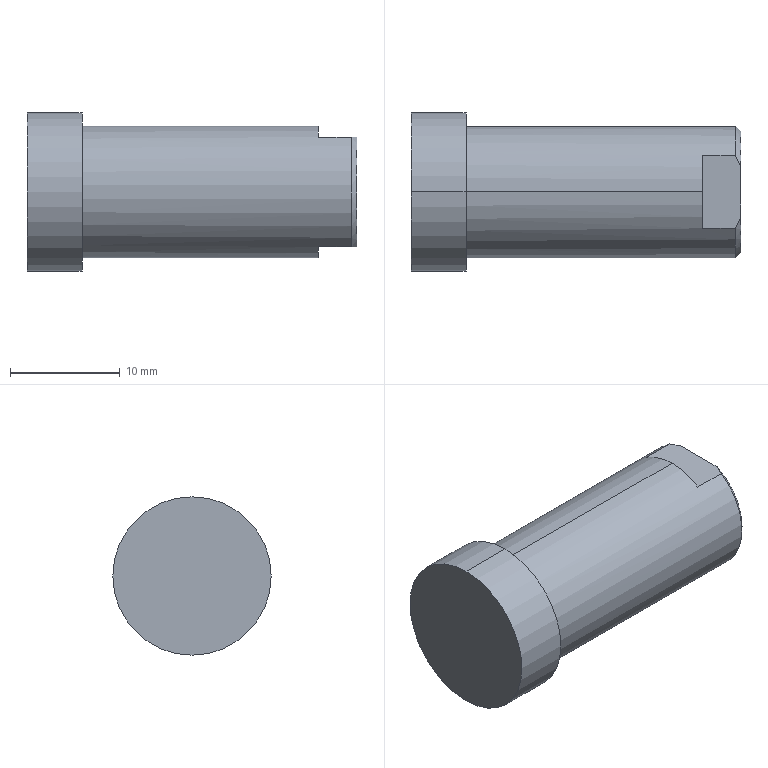Part | STEP file | _MSCCN25-15_rod_1 | 1 solid | 18 faces | box 30 x 14.4 x 14.4 mm | volume 3377 mm3 | plane 8 | cylinder 6 | cone 4 | commonest cylinder face diameters 4.917 x2 12 x2 14.4 x2
STEP:
#1=CARTESIAN_POINT('',(0.,0.,0.));
#2=DIRECTION('',(0.,0.,1.));
#3=DIRECTION('',(1.,0.,0.));
#4=AXIS2_PLACEMENT_3D('',#1,#2,#3);
#5=CARTESIAN_POINT('',(5.,0.,-6.));
#6=VERTEX_POINT('',#5);
#7=CARTESIAN_POINT('',(5.,0.,6.));
#8=VERTEX_POINT('',#7);
#9=CARTESIAN_POINT('',(5.,0.,0.));
#10=DIRECTION('',(1.,0.,0.));
#11=DIRECTION('',(0.,0.,-1.));
#12=AXIS2_PLACEMENT_3D('',#9,#10,#11);
#13=CIRCLE('',#12,6.);
#14=CARTESIAN_POINT('',(30.,0.,0.));
#15=DIRECTION('',(1.,0.,0.));
#16=DIRECTION('',(0.,0.,-1.));
#17=AXIS2_PLACEMENT_3D('',#14,#15,#16);
#18=CYLINDRICAL_SURFACE('',#17,6.);
#19=CARTESIAN_POINT('',(0.,-25.));
#20=DIRECTION('',(1.,0.));
#21=VECTOR('',#20,1.);
#22=LINE('',#19,#21);
#23=(GEOMETRIC_REPRESENTATION_CONTEXT(2)PARAMETRIC_REPRESENTATION_CONTEXT()REPRESENTATION_CONTEXT('',''));
#24=DEFINITIONAL_REPRESENTATION('',(#22),#23);
#25=PCURVE('',#18,#24);
#26=CARTESIAN_POINT('',(5.,7.2,0.));
#27=DIRECTION('',(-1.,0.,0.));
#28=DIRECTION('',(0.,0.,1.));
#29=AXIS2_PLACEMENT_3D('',#26,#27,#28);
#30=PLANE('',#29);
#31=CARTESIAN_POINT('',(-6.,-7.2));
#32=CARTESIAN_POINT('',(-6.,3.192));
#33=CARTESIAN_POINT('',(3.,-2.004));
#34=CARTESIAN_POINT('',(12.,-7.2));
#35=CARTESIAN_POINT('',(3.,-12.396));
#36=CARTESIAN_POINT('',(-6.,-17.592));
#37=CARTESIAN_POINT('',(-6.,-7.2));
#38=(BOUNDED_CURVE()B_SPLINE_CURVE(2,(#31,#32,#33,#34,#35,#36,#37),.UNSPECIFIED.,.T.,.F.)B_SPLINE_CURVE_WITH_KNOTS((1,2,2,2,2,1),(-2.094,0.,2.094,4.189,6.283,8.378),.UNSPECIFIED.)CURVE()GEOMETRIC_REPRESENTATION_ITEM()RATIONAL_B_SPLINE_CURVE((1.,0.5,1.,0.5,1.,0.5,1.))REPRESENTATION_ITEM(''));
#39=(GEOMETRIC_REPRESENTATION_CONTEXT(2)PARAMETRIC_REPRESENTATION_CONTEXT()REPRESENTATION_CONTEXT('',''));
#40=DEFINITIONAL_REPRESENTATION('',(#38),#39);
#41=PCURVE('',#30,#40);
#42=SURFACE_CURVE('',#13,(#25,#41),.PCURVE_S1.);
#43=EDGE_CURVE('',#6,#8,#42,.T.);
#44=ORIENTED_EDGE('',*,*,#43,.T.);
#45=CARTESIAN_POINT('',(26.5,0.,6.));
#46=VERTEX_POINT('',#45);
#47=CARTESIAN_POINT('',(30.,0.,6.));
#48=DIRECTION('',(1.,0.,0.));
#49=VECTOR('',#48,1.);
#50=LINE('',#47,#49);
#51=CARTESIAN_POINT('',(3.142,0.));
#52=DIRECTION('',(0.,1.));
#53=VECTOR('',#52,1.);
#54=LINE('',#51,#53);
#55=(GEOMETRIC_REPRESENTATION_CONTEXT(2)PARAMETRIC_REPRESENTATION_CONTEXT()REPRESENTATION_CONTEXT('',''));
#56=DEFINITIONAL_REPRESENTATION('',(#54),#55);
#57=PCURVE('',#18,#56);
#58=CARTESIAN_POINT('',(30.,0.,0.));
#59=DIRECTION('',(1.,0.,0.));
#60=DIRECTION('',(0.,0.,-1.));
#61=AXIS2_PLACEMENT_3D('',#58,#59,#60);
#62=CYLINDRICAL_SURFACE('',#61,6.);
#63=CARTESIAN_POINT('',(3.142,0.));
#64=DIRECTION('',(0.,1.));
#65=VECTOR('',#64,1.);
#66=LINE('',#63,#65);
#67=(GEOMETRIC_REPRESENTATION_CONTEXT(2)PARAMETRIC_REPRESENTATION_CONTEXT()REPRESENTATION_CONTEXT('',''));
#68=DEFINITIONAL_REPRESENTATION('',(#66),#67);
#69=PCURVE('',#62,#68);
#70=SURFACE_CURVE('',#50,(#57,#69),.PCURVE_S1.);
#71=EDGE_CURVE('',#8,#46,#70,.T.);
#72=ORIENTED_EDGE('',*,*,#71,.T.);
#73=CARTESIAN_POINT('',(26.5,3.317,5.));
#74=VERTEX_POINT('',#73);
#75=CARTESIAN_POINT('',(26.5,0.,0.));
#76=DIRECTION('',(-1.,0.,0.));
#77=DIRECTION('',(0.,0.,-1.));
#78=AXIS2_PLACEMENT_3D('',#75,#76,#77);
#79=CIRCLE('',#78,6.);
#80=CARTESIAN_POINT('',(6.283,-3.5));
#81=DIRECTION('',(-1.,0.));
#82=VECTOR('',#81,1.);
#83=LINE('',#80,#82);
#84=(GEOMETRIC_REPRESENTATION_CONTEXT(2)PARAMETRIC_REPRESENTATION_CONTEXT()REPRESENTATION_CONTEXT('',''));
#85=DEFINITIONAL_REPRESENTATION('',(#83),#84);
#86=PCURVE('',#18,#85);
#87=CARTESIAN_POINT('',(26.5,0.,0.));
#88=DIRECTION('',(1.,0.,0.));
#89=DIRECTION('',(0.,0.,-1.));
#90=AXIS2_PLACEMENT_3D('',#87,#88,#89);
#91=PLANE('',#90);
#92=CARTESIAN_POINT('',(6.,0.));
#93=CARTESIAN_POINT('',(6.,-10.392));
#94=CARTESIAN_POINT('',(-3.,-5.196));
#95=CARTESIAN_POINT('',(-12.,0.));
#96=CARTESIAN_POINT('',(-3.,5.196));
#97=CARTESIAN_POINT('',(6.,10.392));
#98=CARTESIAN_POINT('',(6.,0.));
#99=(BOUNDED_CURVE()B_SPLINE_CURVE(2,(#92,#93,#94,#95,#96,#97,#98),.UNSPECIFIED.,.T.,.F.)B_SPLINE_CURVE_WITH_KNOTS((1,2,2,2,2,1),(-2.094,0.,2.094,4.189,6.283,8.378),.UNSPECIFIED.)CURVE()GEOMETRIC_REPRESENTATION_ITEM()RATIONAL_B_SPLINE_CURVE((1.,0.5,1.,0.5,1.,0.5,1.))REPRESENTATION_ITEM(''));
#100=(GEOMETRIC_REPRESENTATION_CONTEXT(2)PARAMETRIC_REPRESENTATION_CONTEXT()REPRESENTATION_CONTEXT('',''));
#101=DEFINITIONAL_REPRESENTATION('',(#99),#100);
#102=PCURVE('',#91,#101);
#103=SURFACE_CURVE('',#79,(#86,#102),.PCURVE_S1.);
#104=EDGE_CURVE('',#46,#74,#103,.T.);
#105=ORIENTED_EDGE('',*,*,#104,.T.);
#106=CARTESIAN_POINT('',(29.5,3.317,5.));
#107=VERTEX_POINT('',#106);
#108=CARTESIAN_POINT('',(30.,3.317,5.));
#109=DIRECTION('',(1.,0.,0.));
#110=VECTOR('',#109,1.);
#111=LINE('',#108,#110);
#112=CARTESIAN_POINT('',(2.556,0.));
#113=DIRECTION('',(0.,1.));
#114=VECTOR('',#113,1.);
#115=LINE('',#112,#114);
#116=(GEOMETRIC_REPRESENTATION_CONTEXT(2)PARAMETRIC_REPRESENTATION_CONTEXT()REPRESENTATION_CONTEXT('',''));
#117=DEFINITIONAL_REPRESENTATION('',(#115),#116);
#118=PCURVE('',#18,#117);
#119=CARTESIAN_POINT('',(26.5,3.317,5.));
#120=DIRECTION('',(0.,0.,1.));
#121=DIRECTION('',(1.,0.,0.));
#122=AXIS2_PLACEMENT_3D('',#119,#120,#121);
#123=PLANE('',#122);
#124=CARTESIAN_POINT('',(3.5,0.));
#125=DIRECTION('',(1.,0.));
#126=VECTOR('',#125,1.);
#127=LINE('',#124,#126);
#128=(GEOMETRIC_REPRESENTATION_CONTEXT(2)PARAMETRIC_REPRESENTATION_CONTEXT()REPRESENTATION_CONTEXT('',''));
#129=DEFINITIONAL_REPRESENTATION('',(#127),#128);
#130=PCURVE('',#123,#129);
#131=SURFACE_CURVE('',#111,(#118,#130),.PCURVE_S1.);
#132=EDGE_CURVE('',#74,#107,#131,.T.);
#133=ORIENTED_EDGE('',*,*,#132,.T.);
#134=CARTESIAN_POINT('',(29.5,3.317,-5.));
#135=VERTEX_POINT('',#134);
#136=CARTESIAN_POINT('',(29.5,0.,0.));
#137=DIRECTION('',(-1.,0.,0.));
#138=DIRECTION('',(0.,0.,-1.));
#139=AXIS2_PLACEMENT_3D('',#136,#137,#138);
#140=CIRCLE('',#139,6.);
#141=CARTESIAN_POINT('',(6.283,-0.5));
#142=DIRECTION('',(-1.,0.));
#143=VECTOR('',#142,1.);
#144=LINE('',#141,#143);
#145=(GEOMETRIC_REPRESENTATION_CONTEXT(2)PARAMETRIC_REPRESENTATION_CONTEXT()REPRESENTATION_CONTEXT('',''));
#146=DEFINITIONAL_REPRESENTATION('',(#144),#145);
#147=PCURVE('',#18,#146);
#148=CARTESIAN_POINT('',(29.5,0.,0.));
#149=DIRECTION('',(-1.,0.,0.));
#150=DIRECTION('',(0.,0.,1.));
#151=AXIS2_PLACEMENT_3D('',#148,#149,#150);
#152=CONICAL_SURFACE('',#151,6.,0.7854);
#153=CARTESIAN_POINT('',(-3.142,0.));
#154=DIRECTION('',(1.,0.));
#155=VECTOR('',#154,1.);
#156=LINE('',#153,#155);
#157=(GEOMETRIC_REPRESENTATION_CONTEXT(2)PARAMETRIC_REPRESENTATION_CONTEXT()REPRESENTATION_CONTEXT('',''));
#158=DEFINITIONAL_REPRESENTATION('',(#156),#157);
#159=PCURVE('',#152,#158);
#160=SURFACE_CURVE('',#140,(#147,#159),.PCURVE_S1.);
#161=EDGE_CURVE('',#107,#135,#160,.T.);
#162=ORIENTED_EDGE('',*,*,#161,.T.);
#163=CARTESIAN_POINT('',(26.5,3.317,-5.));
#164=VERTEX_POINT('',#163);
#165=CARTESIAN_POINT('',(30.,3.317,-5.));
#166=DIRECTION('',(-1.,0.,0.));
#167=VECTOR('',#166,1.);
#168=LINE('',#165,#167);
#169=CARTESIAN_POINT('',(0.5857,0.));
#170=DIRECTION('',(0.,-1.));
#171=VECTOR('',#170,1.);
#172=LINE('',#169,#171);
#173=(GEOMETRIC_REPRESENTATION_CONTEXT(2)PARAMETRIC_REPRESENTATION_CONTEXT()REPRESENTATION_CONTEXT('',''));
#174=DEFINITIONAL_REPRESENTATION('',(#172),#173);
#175=PCURVE('',#18,#174);
#176=CARTESIAN_POINT('',(26.5,-3.317,-5.));
#177=DIRECTION('',(0.,0.,-1.));
#178=DIRECTION('',(-1.,0.,0.));
#179=AXIS2_PLACEMENT_3D('',#176,#177,#178);
#180=PLANE('',#179);
#181=CARTESIAN_POINT('',(-3.5,6.633));
#182=DIRECTION('',(1.,0.));
#183=VECTOR('',#182,1.);
#184=LINE('',#181,#183);
#185=(GEOMETRIC_REPRESENTATION_CONTEXT(2)PARAMETRIC_REPRESENTATION_CONTEXT()REPRESENTATION_CONTEXT('',''));
#186=DEFINITIONAL_REPRESENTATION('',(#184),#185);
#187=PCURVE('',#180,#186);
#188=SURFACE_CURVE('',#168,(#175,#187),.PCURVE_S1.);
#189=EDGE_CURVE('',#135,#164,#188,.T.);
#190=ORIENTED_EDGE('',*,*,#189,.T.);
#191=CARTESIAN_POINT('',(26.5,0.,-6.));
#192=VERTEX_POINT('',#191);
#193=CARTESIAN_POINT('',(26.5,0.,0.));
#194=DIRECTION('',(-1.,0.,0.));
#195=DIRECTION('',(0.,0.,-1.));
#196=AXIS2_PLACEMENT_3D('',#193,#194,#195);
#197=CIRCLE('',#196,6.);
#198=CARTESIAN_POINT('',(6.283,-3.5));
#199=DIRECTION('',(-1.,0.));
#200=VECTOR('',#199,1.);
#201=LINE('',#198,#200);
#202=(GEOMETRIC_REPRESENTATION_CONTEXT(2)PARAMETRIC_REPRESENTATION_CONTEXT()REPRESENTATION_CONTEXT('',''));
#203=DEFINITIONAL_REPRESENTATION('',(#201),#202);
#204=PCURVE('',#18,#203);
#205=CARTESIAN_POINT('',(26.5,0.,0.));
#206=DIRECTION('',(1.,0.,0.));
#207=DIRECTION('',(0.,0.,-1.));
#208=AXIS2_PLACEMENT_3D('',#205,#206,#207);
#209=PLANE('',#208);
#210=CARTESIAN_POINT('',(6.,0.));
#211=CARTESIAN_POINT('',(6.,-10.392));
#212=CARTESIAN_POINT('',(-3.,-5.196));
#213=CARTESIAN_POINT('',(-12.,0.));
#214=CARTESIAN_POINT('',(-3.,5.196));
#215=CARTESIAN_POINT('',(6.,10.392));
#216=CARTESIAN_POINT('',(6.,0.));
#217=(BOUNDED_CURVE()B_SPLINE_CURVE(2,(#210,#211,#212,#213,#214,#215,#216),.UNSPECIFIED.,.T.,.F.)B_SPLINE_CURVE_WITH_KNOTS((1,2,2,2,2,1),(-2.094,0.,2.094,4.189,6.283,8.378),.UNSPECIFIED.)CURVE()GEOMETRIC_REPRESENTATION_ITEM()RATIONAL_B_SPLINE_CURVE((1.,0.5,1.,0.5,1.,0.5,1.))REPRESENTATION_ITEM(''));
#218=(GEOMETRIC_REPRESENTATION_CONTEXT(2)PARAMETRIC_REPRESENTATION_CONTEXT()REPRESENTATION_CONTEXT('',''));
#219=DEFINITIONAL_REPRESENTATION('',(#217),#218);
#220=PCURVE('',#209,#219);
#221=SURFACE_CURVE('',#197,(#204,#220),.PCURVE_S1.);
#222=EDGE_CURVE('',#164,#192,#221,.T.);
#223=ORIENTED_EDGE('',*,*,#222,.T.);
#224=CARTESIAN_POINT('',(30.,0.,-6.));
#225=DIRECTION('',(1.,0.,0.));
#226=VECTOR('',#225,1.);
#227=LINE('',#224,#226);
#228=CARTESIAN_POINT('',(0.,0.));
#229=DIRECTION('',(0.,1.));
#230=VECTOR('',#229,1.);
#231=LINE('',#228,#230);
#232=(GEOMETRIC_REPRESENTATION_CONTEXT(2)PARAMETRIC_REPRESENTATION_CONTEXT()REPRESENTATION_CONTEXT('',''));
#233=DEFINITIONAL_REPRESENTATION('',(#231),#232);
#234=PCURVE('',#18,#233);
#235=CARTESIAN_POINT('',(6.283,0.));
#236=DIRECTION('',(0.,1.));
#237=VECTOR('',#236,1.);
#238=LINE('',#235,#237);
#239=(GEOMETRIC_REPRESENTATION_CONTEXT(2)PARAMETRIC_REPRESENTATION_CONTEXT()REPRESENTATION_CONTEXT('',''));
#240=DEFINITIONAL_REPRESENTATION('',(#238),#239);
#241=PCURVE('',#62,#240);
#242=SURFACE_CURVE('',#227,(#234,#241),.PCURVE_S1.);
#243=EDGE_CURVE('',#6,#192,#242,.T.);
#244=ORIENTED_EDGE('',*,*,#243,.F.);
#245=EDGE_LOOP('',(#44,#72,#105,#133,#162,#190,#223,#244));
#246=FACE_BOUND('',#245,.T.);
#247=ADVANCED_FACE('',(#246),#18,.T.);
#248=CARTESIAN_POINT('',(0.,0.,-7.2));
#249=VERTEX_POINT('',#248);
#250=CARTESIAN_POINT('',(0.,0.,7.2));
#251=VERTEX_POINT('',#250);
#252=CARTESIAN_POINT('',(0.,0.,0.));
#253=DIRECTION('',(1.,0.,0.));
#254=DIRECTION('',(0.,0.,-1.));
#255=AXIS2_PLACEMENT_3D('',#252,#253,#254);
#256=CIRCLE('',#255,7.2);
#257=CARTESIAN_POINT('',(30.,0.,0.));
#258=DIRECTION('',(1.,0.,0.));
#259=DIRECTION('',(0.,0.,-1.));
#260=AXIS2_PLACEMENT_3D('',#257,#258,#259);
#261=CYLINDRICAL_SURFACE('',#260,7.2);
#262=CARTESIAN_POINT('',(0.,-30.));
#263=DIRECTION('',(1.,0.));
#264=VECTOR('',#263,1.);
#265=LINE('',#262,#264);
#266=(GEOMETRIC_REPRESENTATION_CONTEXT(2)PARAMETRIC_REPRESENTATION_CONTEXT()REPRESENTATION_CONTEXT('',''));
#267=DEFINITIONAL_REPRESENTATION('',(#265),#266);
#268=PCURVE('',#261,#267);
#269=CARTESIAN_POINT('',(0.,0.,0.));
#270=DIRECTION('',(1.,0.,0.));
#271=DIRECTION('',(0.,0.,-1.));
#272=AXIS2_PLACEMENT_3D('',#269,#270,#271);
#273=PLANE('',#272);
#274=CARTESIAN_POINT('',(0.,0.));
#275=DIRECTION('',(1.,0.));
#276=AXIS2_PLACEMENT_2D('',#274,#275);
#277=CIRCLE('',#276,7.2);
#278=(GEOMETRIC_REPRESENTATION_CONTEXT(2)PARAMETRIC_REPRESENTATION_CONTEXT()REPRESENTATION_CONTEXT('',''));
#279=DEFINITIONAL_REPRESENTATION('',(#277),#278);
#280=PCURVE('',#273,#279);
#281=SURFACE_CURVE('',#256,(#268,#280),.PCURVE_S1.);
#282=EDGE_CURVE('',#249,#251,#281,.T.);
#283=ORIENTED_EDGE('',*,*,#282,.T.);
#284=CARTESIAN_POINT('',(5.,0.,7.2));
#285=VERTEX_POINT('',#284);
#286=CARTESIAN_POINT('',(30.,0.,7.2));
#287=DIRECTION('',(1.,0.,0.));
#288=VECTOR('',#287,1.);
#289=LINE('',#286,#288);
#290=CARTESIAN_POINT('',(3.142,0.));
#291=DIRECTION('',(0.,1.));
#292=VECTOR('',#291,1.);
#293=LINE('',#290,#292);
#294=(GEOMETRIC_REPRESENTATION_CONTEXT(2)PARAMETRIC_REPRESENTATION_CONTEXT()REPRESENTATION_CONTEXT('',''));
#295=DEFINITIONAL_REPRESENTATION('',(#293),#294);
#296=PCURVE('',#261,#295);
#297=CARTESIAN_POINT('',(30.,0.,0.));
#298=DIRECTION('',(1.,0.,0.));
#299=DIRECTION('',(0.,0.,-1.));
#300=AXIS2_PLACEMENT_3D('',#297,#298,#299);
#301=CYLINDRICAL_SURFACE('',#300,7.2);
#302=CARTESIAN_POINT('',(3.142,0.));
#303=DIRECTION('',(0.,1.));
#304=VECTOR('',#303,1.);
#305=LINE('',#302,#304);
#306=(GEOMETRIC_REPRESENTATION_CONTEXT(2)PARAMETRIC_REPRESENTATION_CONTEXT()REPRESENTATION_CONTEXT('',''));
#307=DEFINITIONAL_REPRESENTATION('',(#305),#306);
#308=PCURVE('',#301,#307);
#309=SURFACE_CURVE('',#289,(#296,#308),.PCURVE_S1.);
#310=EDGE_CURVE('',#251,#285,#309,.T.);
#311=ORIENTED_EDGE('',*,*,#310,.T.);
#312=CARTESIAN_POINT('',(5.,0.,-7.2));
#313=VERTEX_POINT('',#312);
#314=CARTESIAN_POINT('',(5.,0.,0.));
#315=DIRECTION('',(-1.,0.,0.));
#316=DIRECTION('',(0.,0.,-1.));
#317=AXIS2_PLACEMENT_3D('',#314,#315,#316);
#318=CIRCLE('',#317,7.2);
#319=CARTESIAN_POINT('',(6.283,-25.));
#320=DIRECTION('',(-1.,0.));
#321=VECTOR('',#320,1.);
#322=LINE('',#319,#321);
#323=(GEOMETRIC_REPRESENTATION_CONTEXT(2)PARAMETRIC_REPRESENTATION_CONTEXT()REPRESENTATION_CONTEXT('',''));
#324=DEFINITIONAL_REPRESENTATION('',(#322),#323);
#325=PCURVE('',#261,#324);
#326=CARTESIAN_POINT('',(0.,-7.2));
#327=DIRECTION('',(-1.,0.));
#328=AXIS2_PLACEMENT_2D('',#326,#327);
#329=CIRCLE('',#328,7.2);
#330=(GEOMETRIC_REPRESENTATION_CONTEXT(2)PARAMETRIC_REPRESENTATION_CONTEXT()REPRESENTATION_CONTEXT('',''));
#331=DEFINITIONAL_REPRESENTATION('',(#329),#330);
#332=PCURVE('',#30,#331);
#333=SURFACE_CURVE('',#318,(#325,#332),.PCURVE_S1.);
#334=EDGE_CURVE('',#285,#313,#333,.T.);
#335=ORIENTED_EDGE('',*,*,#334,.T.);
#336=CARTESIAN_POINT('',(30.,0.,-7.2));
#337=DIRECTION('',(1.,0.,0.));
#338=VECTOR('',#337,1.);
#339=LINE('',#336,#338);
#340=CARTESIAN_POINT('',(0.,0.));
#341=DIRECTION('',(0.,1.));
#342=VECTOR('',#341,1.);
#343=LINE('',#340,#342);
#344=(GEOMETRIC_REPRESENTATION_CONTEXT(2)PARAMETRIC_REPRESENTATION_CONTEXT()REPRESENTATION_CONTEXT('',''));
#345=DEFINITIONAL_REPRESENTATION('',(#343),#344);
#346=PCURVE('',#261,#345);
#347=CARTESIAN_POINT('',(6.283,0.));
#348=DIRECTION('',(0.,1.));
#349=VECTOR('',#348,1.);
#350=LINE('',#347,#349);
#351=(GEOMETRIC_REPRESENTATION_CONTEXT(2)PARAMETRIC_REPRESENTATION_CONTEXT()REPRESENTATION_CONTEXT('',''));
#352=DEFINITIONAL_REPRESENTATION('',(#350),#351);
#353=PCURVE('',#301,#352);
#354=SURFACE_CURVE('',#339,(#346,#353),.PCURVE_S1.);
#355=EDGE_CURVE('',#249,#313,#354,.T.);
#356=ORIENTED_EDGE('',*,*,#355,.F.);
#357=EDGE_LOOP('',(#283,#311,#335,#356));
#358=FACE_BOUND('',#357,.T.);
#359=ADVANCED_FACE('',(#358),#261,.T.);
#360=CARTESIAN_POINT('',(29.459,0.,-2.458));
#361=VERTEX_POINT('',#360);
#362=CARTESIAN_POINT('',(29.459,2.458,0.));
#363=VERTEX_POINT('',#362);
#364=CARTESIAN_POINT('',(29.459,0.,0.));
#365=DIRECTION('',(1.,0.,0.));
#366=DIRECTION('',(0.,0.,-1.));
#367=AXIS2_PLACEMENT_3D('',#364,#365,#366);
#368=CIRCLE('',#367,2.458);
#369=CARTESIAN_POINT('',(30.,0.,0.));
#370=DIRECTION('',(1.,0.,0.));
#371=DIRECTION('',(0.,1.,0.));
#372=AXIS2_PLACEMENT_3D('',#369,#370,#371);
#373=CONICAL_SURFACE('',#372,3.,0.7854);
#374=CARTESIAN_POINT('',(4.712,-0.5415));
#375=DIRECTION('',(1.,0.));
#376=VECTOR('',#375,1.);
#377=LINE('',#374,#376);
#378=(GEOMETRIC_REPRESENTATION_CONTEXT(2)PARAMETRIC_REPRESENTATION_CONTEXT()REPRESENTATION_CONTEXT('',''));
#379=DEFINITIONAL_REPRESENTATION('',(#377),#378);
#380=PCURVE('',#373,#379);
#381=CARTESIAN_POINT('',(30.,0.,0.));
#382=DIRECTION('',(1.,0.,0.));
#383=DIRECTION('',(0.,0.,-1.));
#384=AXIS2_PLACEMENT_3D('',#381,#382,#383);
#385=CYLINDRICAL_SURFACE('',#384,2.458);
#386=CARTESIAN_POINT('',(0.,-0.5415));
#387=DIRECTION('',(1.,0.));
#388=VECTOR('',#387,1.);
#389=LINE('',#386,#388);
#390=(GEOMETRIC_REPRESENTATION_CONTEXT(2)PARAMETRIC_REPRESENTATION_CONTEXT()REPRESENTATION_CONTEXT('',''));
#391=DEFINITIONAL_REPRESENTATION('',(#389),#390);
#392=PCURVE('',#385,#391);
#393=SURFACE_CURVE('',#368,(#380,#392),.PCURVE_S1.);
#394=EDGE_CURVE('',#361,#363,#393,.T.);
#395=ORIENTED_EDGE('',*,*,#394,.T.);
#396=CARTESIAN_POINT('',(30.,3.,0.));
#397=VERTEX_POINT('',#396);
#398=CARTESIAN_POINT('',(30.,3.,0.));
#399=DIRECTION('',(0.7071,0.7071,0.));
#400=VECTOR('',#399,1.);
#401=LINE('',#398,#400);
#402=CARTESIAN_POINT('',(6.283,0.));
#403=DIRECTION('',(0.,1.));
#404=VECTOR('',#403,1.);
#405=LINE('',#402,#404);
#406=(GEOMETRIC_REPRESENTATION_CONTEXT(2)PARAMETRIC_REPRESENTATION_CONTEXT()REPRESENTATION_CONTEXT('',''));
#407=DEFINITIONAL_REPRESENTATION('',(#405),#406);
#408=PCURVE('',#373,#407);
#409=CARTESIAN_POINT('',(30.,0.,0.));
#410=DIRECTION('',(1.,0.,0.));
#411=DIRECTION('',(0.,1.,0.));
#412=AXIS2_PLACEMENT_3D('',#409,#410,#411);
#413=CONICAL_SURFACE('',#412,3.,0.7854);
#414=CARTESIAN_POINT('',(0.,0.));
#415=DIRECTION('',(0.,1.));
#416=VECTOR('',#415,1.);
#417=LINE('',#414,#416);
#418=(GEOMETRIC_REPRESENTATION_CONTEXT(2)PARAMETRIC_REPRESENTATION_CONTEXT()REPRESENTATION_CONTEXT('',''));
#419=DEFINITIONAL_REPRESENTATION('',(#417),#418);
#420=PCURVE('',#413,#419);
#421=SURFACE_CURVE('',#401,(#408,#420),.PCURVE_S1.);
#422=EDGE_CURVE('',#363,#397,#421,.T.);
#423=ORIENTED_EDGE('',*,*,#422,.T.);
#424=CARTESIAN_POINT('',(30.,-3.,0.));
#425=VERTEX_POINT('',#424);
#426=CARTESIAN_POINT('',(30.,0.,0.));
#427=DIRECTION('',(1.,0.,0.));
#428=DIRECTION('',(0.,1.,0.));
#429=AXIS2_PLACEMENT_3D('',#426,#427,#428);
#430=CIRCLE('',#429,3.);
#431=CARTESIAN_POINT('',(0.,0.));
#432=DIRECTION('',(1.,0.));
#433=VECTOR('',#432,1.);
#434=LINE('',#431,#433);
#435=(GEOMETRIC_REPRESENTATION_CONTEXT(2)PARAMETRIC_REPRESENTATION_CONTEXT()REPRESENTATION_CONTEXT('',''));
#436=DEFINITIONAL_REPRESENTATION('',(#434),#435);
#437=PCURVE('',#373,#436);
#438=CARTESIAN_POINT('',(30.,5.5,0.));
#439=DIRECTION('',(-1.,0.,0.));
#440=DIRECTION('',(0.,0.,1.));
#441=AXIS2_PLACEMENT_3D('',#438,#439,#440);
#442=PLANE('',#441);
#443=CARTESIAN_POINT('',(0.,-2.5));
#444=CARTESIAN_POINT('',(5.196,-2.5));
#445=CARTESIAN_POINT('',(2.598,-7.));
#446=CARTESIAN_POINT('',(0.,-11.5));
#447=CARTESIAN_POINT('',(-2.598,-7.));
#448=CARTESIAN_POINT('',(-5.196,-2.5));
#449=CARTESIAN_POINT('',(0.,-2.5));
#450=(BOUNDED_CURVE()B_SPLINE_CURVE(2,(#443,#444,#445,#446,#447,#448,#449),.UNSPECIFIED.,.T.,.F.)B_SPLINE_CURVE_WITH_KNOTS((1,2,2,2,2,1),(-2.094,0.,2.094,4.189,6.283,8.378),.UNSPECIFIED.)CURVE()GEOMETRIC_REPRESENTATION_ITEM()RATIONAL_B_SPLINE_CURVE((1.,0.5,1.,0.5,1.,0.5,1.))REPRESENTATION_ITEM(''));
#451=(GEOMETRIC_REPRESENTATION_CONTEXT(2)PARAMETRIC_REPRESENTATION_CONTEXT()REPRESENTATION_CONTEXT('',''));
#452=DEFINITIONAL_REPRESENTATION('',(#450),#451);
#453=PCURVE('',#442,#452);
#454=SURFACE_CURVE('',#430,(#437,#453),.PCURVE_S1.);
#455=EDGE_CURVE('',#425,#397,#454,.T.);
#456=ORIENTED_EDGE('',*,*,#455,.F.);
#457=CARTESIAN_POINT('',(29.459,-2.458,0.));
#458=VERTEX_POINT('',#457);
#459=CARTESIAN_POINT('',(30.,-3.,0.));
#460=DIRECTION('',(0.7071,-0.7071,0.));
#461=VECTOR('',#460,1.);
#462=LINE('',#459,#461);
#463=CARTESIAN_POINT('',(3.142,0.));
#464=DIRECTION('',(0.,1.));
#465=VECTOR('',#464,1.);
#466=LINE('',#463,#465);
#467=(GEOMETRIC_REPRESENTATION_CONTEXT(2)PARAMETRIC_REPRESENTATION_CONTEXT()REPRESENTATION_CONTEXT('',''));
#468=DEFINITIONAL_REPRESENTATION('',(#466),#467);
#469=PCURVE('',#373,#468);
#470=CARTESIAN_POINT('',(3.142,0.));
#471=DIRECTION('',(0.,1.));
#472=VECTOR('',#471,1.);
#473=LINE('',#470,#472);
#474=(GEOMETRIC_REPRESENTATION_CONTEXT(2)PARAMETRIC_REPRESENTATION_CONTEXT()REPRESENTATION_CONTEXT('',''));
#475=DEFINITIONAL_REPRESENTATION('',(#473),#474);
#476=PCURVE('',#413,#475);
#477=SURFACE_CURVE('',#462,(#469,#476),.PCURVE_S1.);
#478=EDGE_CURVE('',#458,#425,#477,.T.);
#479=ORIENTED_EDGE('',*,*,#478,.F.);
#480=CARTESIAN_POINT('',(29.459,0.,0.));
#481=DIRECTION('',(1.,0.,0.));
#482=DIRECTION('',(0.,0.,-1.));
#483=AXIS2_PLACEMENT_3D('',#480,#481,#482);
#484=CIRCLE('',#483,2.458);
#485=CARTESIAN_POINT('',(-1.571,-0.5415));
#486=DIRECTION('',(1.,0.));
#487=VECTOR('',#486,1.);
#488=LINE('',#485,#487);
#489=(GEOMETRIC_REPRESENTATION_CONTEXT(2)PARAMETRIC_REPRESENTATION_CONTEXT()REPRESENTATION_CONTEXT('',''));
#490=DEFINITIONAL_REPRESENTATION('',(#488),#489);
#491=PCURVE('',#373,#490);
#492=CARTESIAN_POINT('',(30.,0.,0.));
#493=DIRECTION('',(1.,0.,0.));
#494=DIRECTION('',(0.,0.,-1.));
#495=AXIS2_PLACEMENT_3D('',#492,#493,#494);
#496=CYLINDRICAL_SURFACE('',#495,2.458);
#497=CARTESIAN_POINT('',(0.,-0.5415));
#498=DIRECTION('',(1.,0.));
#499=VECTOR('',#498,1.);
#500=LINE('',#497,#499);
#501=(GEOMETRIC_REPRESENTATION_CONTEXT(2)PARAMETRIC_REPRESENTATION_CONTEXT()REPRESENTATION_CONTEXT('',''));
#502=DEFINITIONAL_REPRESENTATION('',(#500),#501);
#503=PCURVE('',#496,#502);
#504=SURFACE_CURVE('',#484,(#491,#503),.PCURVE_S1.);
#505=EDGE_CURVE('',#458,#361,#504,.T.);
#506=ORIENTED_EDGE('',*,*,#505,.T.);
#507=EDGE_LOOP('',(#395,#423,#456,#479,#506));
#508=FACE_BOUND('',#507,.F.);
#509=ADVANCED_FACE('',(#508),#373,.F.);
#510=CARTESIAN_POINT('',(18.,0.,-2.458));
#511=VERTEX_POINT('',#510);
#512=CARTESIAN_POINT('',(30.,0.,-2.458));
#513=DIRECTION('',(1.,0.,0.));
#514=VECTOR('',#513,1.);
#515=LINE('',#512,#514);
#516=CARTESIAN_POINT('',(6.283,0.));
#517=DIRECTION('',(0.,1.));
#518=VECTOR('',#517,1.);
#519=LINE('',#516,#518);
#520=(GEOMETRIC_REPRESENTATION_CONTEXT(2)PARAMETRIC_REPRESENTATION_CONTEXT()REPRESENTATION_CONTEXT('',''));
#521=DEFINITIONAL_REPRESENTATION('',(#519),#520);
#522=PCURVE('',#496,#521);
#523=CARTESIAN_POINT('',(0.,0.));
#524=DIRECTION('',(0.,1.));
#525=VECTOR('',#524,1.);
#526=LINE('',#523,#525);
#527=(GEOMETRIC_REPRESENTATION_CONTEXT(2)PARAMETRIC_REPRESENTATION_CONTEXT()REPRESENTATION_CONTEXT('',''));
#528=DEFINITIONAL_REPRESENTATION('',(#526),#527);
#529=PCURVE('',#385,#528);
#530=SURFACE_CURVE('',#515,(#522,#529),.PCURVE_S1.);
#531=EDGE_CURVE('',#511,#361,#530,.T.);
#532=ORIENTED_EDGE('',*,*,#531,.T.);
#533=ORIENTED_EDGE('',*,*,#505,.F.);
#534=CARTESIAN_POINT('',(29.459,0.,2.458));
#535=VERTEX_POINT('',#534);
#536=CARTESIAN_POINT('',(29.459,0.,0.));
#537=DIRECTION('',(1.,0.,0.));
#538=DIRECTION('',(0.,0.,-1.));
#539=AXIS2_PLACEMENT_3D('',#536,#537,#538);
#540=CIRCLE('',#539,2.458);
#541=CARTESIAN_POINT('',(0.,-0.5415));
#542=DIRECTION('',(1.,0.));
#543=VECTOR('',#542,1.);
#544=LINE('',#541,#543);
#545=(GEOMETRIC_REPRESENTATION_CONTEXT(2)PARAMETRIC_REPRESENTATION_CONTEXT()REPRESENTATION_CONTEXT('',''));
#546=DEFINITIONAL_REPRESENTATION('',(#544),#545);
#547=PCURVE('',#496,#546);
#548=CARTESIAN_POINT('',(-1.571,-0.5415));
#549=DIRECTION('',(1.,0.));
#550=VECTOR('',#549,1.);
#551=LINE('',#548,#550);
#552=(GEOMETRIC_REPRESENTATION_CONTEXT(2)PARAMETRIC_REPRESENTATION_CONTEXT()REPRESENTATION_CONTEXT('',''));
#553=DEFINITIONAL_REPRESENTATION('',(#551),#552);
#554=PCURVE('',#413,#553);
#555=SURFACE_CURVE('',#540,(#547,#554),.PCURVE_S1.);
#556=EDGE_CURVE('',#535,#458,#555,.T.);
#557=ORIENTED_EDGE('',*,*,#556,.F.);
#558=CARTESIAN_POINT('',(18.,0.,2.458));
#559=VERTEX_POINT('',#558);
#560=CARTESIAN_POINT('',(30.,0.,2.458));
#561=DIRECTION('',(1.,0.,0.));
#562=VECTOR('',#561,1.);
#563=LINE('',#560,#562);
#564=CARTESIAN_POINT('',(3.142,0.));
#565=DIRECTION('',(0.,1.));
#566=VECTOR('',#565,1.);
#567=LINE('',#564,#566);
#568=(GEOMETRIC_REPRESENTATION_CONTEXT(2)PARAMETRIC_REPRESENTATION_CONTEXT()REPRESENTATION_CONTEXT('',''));
#569=DEFINITIONAL_REPRESENTATION('',(#567),#568);
#570=PCURVE('',#496,#569);
#571=CARTESIAN_POINT('',(3.142,0.));
#572=DIRECTION('',(0.,1.));
#573=VECTOR('',#572,1.);
#574=LINE('',#571,#573);
#575=(GEOMETRIC_REPRESENTATION_CONTEXT(2)PARAMETRIC_REPRESENTATION_CONTEXT()REPRESENTATION_CONTEXT('',''));
#576=DEFINITIONAL_REPRESENTATION('',(#574),#575);
#577=PCURVE('',#385,#576);
#578=SURFACE_CURVE('',#563,(#570,#577),.PCURVE_S1.);
#579=EDGE_CURVE('',#559,#535,#578,.T.);
#580=ORIENTED_EDGE('',*,*,#579,.F.);
#581=CARTESIAN_POINT('',(18.,0.,0.));
#582=DIRECTION('',(1.,0.,0.));
#583=DIRECTION('',(0.,0.,-1.));
#584=AXIS2_PLACEMENT_3D('',#581,#582,#583);
#585=CIRCLE('',#584,2.458);
#586=CARTESIAN_POINT('',(0.,-12.));
#587=DIRECTION('',(1.,0.));
#588=VECTOR('',#587,1.);
#589=LINE('',#586,#588);
#590=(GEOMETRIC_REPRESENTATION_CONTEXT(2)PARAMETRIC_REPRESENTATION_CONTEXT()REPRESENTATION_CONTEXT('',''));
#591=DEFINITIONAL_REPRESENTATION('',(#589),#590);
#592=PCURVE('',#496,#591);
#593=CARTESIAN_POINT('',(18.,0.,0.));
#594=DIRECTION('',(1.,0.,0.));
#595=DIRECTION('',(0.,0.,-1.));
#596=AXIS2_PLACEMENT_3D('',#593,#594,#595);
#597=PLANE('',#596);
#598=CARTESIAN_POINT('',(0.,0.));
#599=DIRECTION('',(1.,0.));
#600=AXIS2_PLACEMENT_2D('',#598,#599);
#601=CIRCLE('',#600,2.458);
#602=(GEOMETRIC_REPRESENTATION_CONTEXT(2)PARAMETRIC_REPRESENTATION_CONTEXT()REPRESENTATION_CONTEXT('',''));
#603=DEFINITIONAL_REPRESENTATION('',(#601),#602);
#604=PCURVE('',#597,#603);
#605=SURFACE_CURVE('',#585,(#592,#604),.PCURVE_S1.);
#606=EDGE_CURVE('',#559,#511,#605,.T.);
#607=ORIENTED_EDGE('',*,*,#606,.T.);
#608=EDGE_LOOP('',(#532,#533,#557,#580,#607));
#609=FACE_BOUND('',#608,.F.);
#610=ADVANCED_FACE('',(#609),#496,.F.);
#611=ORIENTED_EDGE('',*,*,#71,.F.);
#612=CARTESIAN_POINT('',(5.,0.,0.));
#613=DIRECTION('',(1.,0.,0.));
#614=DIRECTION('',(0.,0.,-1.));
#615=AXIS2_PLACEMENT_3D('',#612,#613,#614);
#616=CIRCLE('',#615,6.);
#617=CARTESIAN_POINT('',(0.,-25.));
#618=DIRECTION('',(1.,0.));
#619=VECTOR('',#618,1.);
#620=LINE('',#617,#619);
#621=(GEOMETRIC_REPRESENTATION_CONTEXT(2)PARAMETRIC_REPRESENTATION_CONTEXT()REPRESENTATION_CONTEXT('',''));
#622=DEFINITIONAL_REPRESENTATION('',(#620),#621);
#623=PCURVE('',#62,#622);
#624=CARTESIAN_POINT('',(-6.,-7.2));
#625=CARTESIAN_POINT('',(-6.,3.192));
#626=CARTESIAN_POINT('',(3.,-2.004));
#627=CARTESIAN_POINT('',(12.,-7.2));
#628=CARTESIAN_POINT('',(3.,-12.396));
#629=CARTESIAN_POINT('',(-6.,-17.592));
#630=CARTESIAN_POINT('',(-6.,-7.2));
#631=(BOUNDED_CURVE()B_SPLINE_CURVE(2,(#624,#625,#626,#627,#628,#629,#630),.UNSPECIFIED.,.T.,.F.)B_SPLINE_CURVE_WITH_KNOTS((1,2,2,2,2,1),(-2.094,0.,2.094,4.189,6.283,8.378),.UNSPECIFIED.)CURVE()GEOMETRIC_REPRESENTATION_ITEM()RATIONAL_B_SPLINE_CURVE((1.,0.5,1.,0.5,1.,0.5,1.))REPRESENTATION_ITEM(''));
#632=(GEOMETRIC_REPRESENTATION_CONTEXT(2)PARAMETRIC_REPRESENTATION_CONTEXT()REPRESENTATION_CONTEXT('',''));
#633=DEFINITIONAL_REPRESENTATION('',(#631),#632);
#634=PCURVE('',#30,#633);
#635=SURFACE_CURVE('',#616,(#623,#634),.PCURVE_S1.);
#636=EDGE_CURVE('',#8,#6,#635,.T.);
#637=ORIENTED_EDGE('',*,*,#636,.T.);
#638=ORIENTED_EDGE('',*,*,#243,.T.);
#639=CARTESIAN_POINT('',(26.5,-3.317,-5.));
#640=VERTEX_POINT('',#639);
#641=CARTESIAN_POINT('',(26.5,0.,0.));
#642=DIRECTION('',(-1.,0.,0.));
#643=DIRECTION('',(0.,0.,-1.));
#644=AXIS2_PLACEMENT_3D('',#641,#642,#643);
#645=CIRCLE('',#644,6.);
#646=CARTESIAN_POINT('',(6.283,-3.5));
#647=DIRECTION('',(-1.,0.));
#648=VECTOR('',#647,1.);
#649=LINE('',#646,#648);
#650=(GEOMETRIC_REPRESENTATION_CONTEXT(2)PARAMETRIC_REPRESENTATION_CONTEXT()REPRESENTATION_CONTEXT('',''));
#651=DEFINITIONAL_REPRESENTATION('',(#649),#650);
#652=PCURVE('',#62,#651);
#653=CARTESIAN_POINT('',(6.,0.));
#654=CARTESIAN_POINT('',(6.,-10.392));
#655=CARTESIAN_POINT('',(-3.,-5.196));
#656=CARTESIAN_POINT('',(-12.,0.));
#657=CARTESIAN_POINT('',(-3.,5.196));
#658=CARTESIAN_POINT('',(6.,10.392));
#659=CARTESIAN_POINT('',(6.,0.));
#660=(BOUNDED_CURVE()B_SPLINE_CURVE(2,(#653,#654,#655,#656,#657,#658,#659),.UNSPECIFIED.,.T.,.F.)B_SPLINE_CURVE_WITH_KNOTS((1,2,2,2,2,1),(-2.094,0.,2.094,4.189,6.283,8.378),.UNSPECIFIED.)CURVE()GEOMETRIC_REPRESENTATION_ITEM()RATIONAL_B_SPLINE_CURVE((1.,0.5,1.,0.5,1.,0.5,1.))REPRESENTATION_ITEM(''));
#661=(GEOMETRIC_REPRESENTATION_CONTEXT(2)PARAMETRIC_REPRESENTATION_CONTEXT()REPRESENTATION_CONTEXT('',''));
#662=DEFINITIONAL_REPRESENTATION('',(#660),#661);
#663=PCURVE('',#209,#662);
#664=SURFACE_CURVE('',#645,(#652,#663),.PCURVE_S1.);
#665=EDGE_CURVE('',#192,#640,#664,.T.);
#666=ORIENTED_EDGE('',*,*,#665,.T.);
#667=CARTESIAN_POINT('',(29.5,-3.317,-5.));
#668=VERTEX_POINT('',#667);
#669=CARTESIAN_POINT('',(30.,-3.317,-5.));
#670=DIRECTION('',(1.,0.,0.));
#671=VECTOR('',#670,1.);
#672=LINE('',#669,#671);
#673=CARTESIAN_POINT('',(5.697,0.));
#674=DIRECTION('',(0.,1.));
#675=VECTOR('',#674,1.);
#676=LINE('',#673,#675);
#677=(GEOMETRIC_REPRESENTATION_CONTEXT(2)PARAMETRIC_REPRESENTATION_CONTEXT()REPRESENTATION_CONTEXT('',''));
#678=DEFINITIONAL_REPRESENTATION('',(#676),#677);
#679=PCURVE('',#62,#678);
#680=CARTESIAN_POINT('',(-3.5,0.));
#681=DIRECTION('',(-1.,0.));
#682=VECTOR('',#681,1.);
#683=LINE('',#680,#682);
#684=(GEOMETRIC_REPRESENTATION_CONTEXT(2)PARAMETRIC_REPRESENTATION_CONTEXT()REPRESENTATION_CONTEXT('',''));
#685=DEFINITIONAL_REPRESENTATION('',(#683),#684);
#686=PCURVE('',#180,#685);
#687=SURFACE_CURVE('',#672,(#679,#686),.PCURVE_S1.);
#688=EDGE_CURVE('',#640,#668,#687,.T.);
#689=ORIENTED_EDGE('',*,*,#688,.T.);
#690=CARTESIAN_POINT('',(29.5,-3.317,5.));
#691=VERTEX_POINT('',#690);
#692=CARTESIAN_POINT('',(29.5,0.,0.));
#693=DIRECTION('',(-1.,0.,0.));
#694=DIRECTION('',(0.,0.,-1.));
#695=AXIS2_PLACEMENT_3D('',#692,#693,#694);
#696=CIRCLE('',#695,6.);
#697=CARTESIAN_POINT('',(6.283,-0.5));
#698=DIRECTION('',(-1.,0.));
#699=VECTOR('',#698,1.);
#700=LINE('',#697,#699);
#701=(GEOMETRIC_REPRESENTATION_CONTEXT(2)PARAMETRIC_REPRESENTATION_CONTEXT()REPRESENTATION_CONTEXT('',''));
#702=DEFINITIONAL_REPRESENTATION('',(#700),#701);
#703=PCURVE('',#62,#702);
#704=CARTESIAN_POINT('',(29.5,0.,0.));
#705=DIRECTION('',(-1.,0.,0.));
#706=DIRECTION('',(0.,0.,1.));
#707=AXIS2_PLACEMENT_3D('',#704,#705,#706);
#708=CONICAL_SURFACE('',#707,6.,0.7854);
#709=CARTESIAN_POINT('',(3.142,0.));
#710=DIRECTION('',(1.,0.));
#711=VECTOR('',#710,1.);
#712=LINE('',#709,#711);
#713=(GEOMETRIC_REPRESENTATION_CONTEXT(2)PARAMETRIC_REPRESENTATION_CONTEXT()REPRESENTATION_CONTEXT('',''));
#714=DEFINITIONAL_REPRESENTATION('',(#712),#713);
#715=PCURVE('',#708,#714);
#716=SURFACE_CURVE('',#696,(#703,#715),.PCURVE_S1.);
#717=EDGE_CURVE('',#668,#691,#716,.T.);
#718=ORIENTED_EDGE('',*,*,#717,.T.);
#719=CARTESIAN_POINT('',(26.5,-3.317,5.));
#720=VERTEX_POINT('',#719);
#721=CARTESIAN_POINT('',(30.,-3.317,5.));
#722=DIRECTION('',(-1.,0.,0.));
#723=VECTOR('',#722,1.);
#724=LINE('',#721,#723);
#725=CARTESIAN_POINT('',(3.727,0.));
#726=DIRECTION('',(0.,-1.));
#727=VECTOR('',#726,1.);
#728=LINE('',#725,#727);
#729=(GEOMETRIC_REPRESENTATION_CONTEXT(2)PARAMETRIC_REPRESENTATION_CONTEXT()REPRESENTATION_CONTEXT('',''));
#730=DEFINITIONAL_REPRESENTATION('',(#728),#729);
#731=PCURVE('',#62,#730);
#732=CARTESIAN_POINT('',(3.5,-6.633));
#733=DIRECTION('',(-1.,0.));
#734=VECTOR('',#733,1.);
#735=LINE('',#732,#734);
#736=(GEOMETRIC_REPRESENTATION_CONTEXT(2)PARAMETRIC_REPRESENTATION_CONTEXT()REPRESENTATION_CONTEXT('',''));
#737=DEFINITIONAL_REPRESENTATION('',(#735),#736);
#738=PCURVE('',#123,#737);
#739=SURFACE_CURVE('',#724,(#731,#738),.PCURVE_S1.);
#740=EDGE_CURVE('',#691,#720,#739,.T.);
#741=ORIENTED_EDGE('',*,*,#740,.T.);
#742=CARTESIAN_POINT('',(26.5,0.,0.));
#743=DIRECTION('',(-1.,0.,0.));
#744=DIRECTION('',(0.,0.,-1.));
#745=AXIS2_PLACEMENT_3D('',#742,#743,#744);
#746=CIRCLE('',#745,6.);
#747=CARTESIAN_POINT('',(6.283,-3.5));
#748=DIRECTION('',(-1.,0.));
#749=VECTOR('',#748,1.);
#750=LINE('',#747,#749);
#751=(GEOMETRIC_REPRESENTATION_CONTEXT(2)PARAMETRIC_REPRESENTATION_CONTEXT()REPRESENTATION_CONTEXT('',''));
#752=DEFINITIONAL_REPRESENTATION('',(#750),#751);
#753=PCURVE('',#62,#752);
#754=CARTESIAN_POINT('',(6.,0.));
#755=CARTESIAN_POINT('',(6.,-10.392));
#756=CARTESIAN_POINT('',(-3.,-5.196));
#757=CARTESIAN_POINT('',(-12.,0.));
#758=CARTESIAN_POINT('',(-3.,5.196));
#759=CARTESIAN_POINT('',(6.,10.392));
#760=CARTESIAN_POINT('',(6.,0.));
#761=(BOUNDED_CURVE()B_SPLINE_CURVE(2,(#754,#755,#756,#757,#758,#759,#760),.UNSPECIFIED.,.T.,.F.)B_SPLINE_CURVE_WITH_KNOTS((1,2,2,2,2,1),(-2.094,0.,2.094,4.189,6.283,8.378),.UNSPECIFIED.)CURVE()GEOMETRIC_REPRESENTATION_ITEM()RATIONAL_B_SPLINE_CURVE((1.,0.5,1.,0.5,1.,0.5,1.))REPRESENTATION_ITEM(''));
#762=(GEOMETRIC_REPRESENTATION_CONTEXT(2)PARAMETRIC_REPRESENTATION_CONTEXT()REPRESENTATION_CONTEXT('',''));
#763=DEFINITIONAL_REPRESENTATION('',(#761),#762);
#764=PCURVE('',#91,#763);
#765=SURFACE_CURVE('',#746,(#753,#764),.PCURVE_S1.);
#766=EDGE_CURVE('',#720,#46,#765,.T.);
#767=ORIENTED_EDGE('',*,*,#766,.T.);
#768=EDGE_LOOP('',(#611,#637,#638,#666,#689,#718,#741,#767));
#769=FACE_BOUND('',#768,.T.);
#770=ADVANCED_FACE('',(#769),#62,.T.);
#771=ORIENTED_EDGE('',*,*,#43,.F.);
#772=ORIENTED_EDGE('',*,*,#636,.F.);
#773=EDGE_LOOP('',(#771,#772));
#774=FACE_BOUND('',#773,.T.);
#775=CARTESIAN_POINT('',(5.,0.,0.));
#776=DIRECTION('',(-1.,0.,0.));
#777=DIRECTION('',(0.,0.,-1.));
#778=AXIS2_PLACEMENT_3D('',#775,#776,#777);
#779=CIRCLE('',#778,7.2);
#780=CARTESIAN_POINT('',(0.,-7.2));
#781=DIRECTION('',(-1.,0.));
#782=AXIS2_PLACEMENT_2D('',#780,#781);
#783=CIRCLE('',#782,7.2);
#784=(GEOMETRIC_REPRESENTATION_CONTEXT(2)PARAMETRIC_REPRESENTATION_CONTEXT()REPRESENTATION_CONTEXT('',''));
#785=DEFINITIONAL_REPRESENTATION('',(#783),#784);
#786=PCURVE('',#30,#785);
#787=CARTESIAN_POINT('',(6.283,-25.));
#788=DIRECTION('',(-1.,0.));
#789=VECTOR('',#788,1.);
#790=LINE('',#787,#789);
#791=(GEOMETRIC_REPRESENTATION_CONTEXT(2)PARAMETRIC_REPRESENTATION_CONTEXT()REPRESENTATION_CONTEXT('',''));
#792=DEFINITIONAL_REPRESENTATION('',(#790),#791);
#793=PCURVE('',#301,#792);
#794=SURFACE_CURVE('',#779,(#786,#793),.PCURVE_S1.);
#795=EDGE_CURVE('',#313,#285,#794,.T.);
#796=ORIENTED_EDGE('',*,*,#795,.F.);
#797=ORIENTED_EDGE('',*,*,#334,.F.);
#798=EDGE_LOOP('',(#796,#797));
#799=FACE_BOUND('',#798,.T.);
#800=ADVANCED_FACE('',(#774,#799),#30,.F.);
#801=CARTESIAN_POINT('',(26.5,0.,-5.));
#802=DIRECTION('',(0.,-1.,0.));
#803=VECTOR('',#802,1.);
#804=LINE('',#801,#803);
#805=CARTESIAN_POINT('',(5.,0.));
#806=DIRECTION('',(0.,-1.));
#807=VECTOR('',#806,1.);
#808=LINE('',#805,#807);
#809=(GEOMETRIC_REPRESENTATION_CONTEXT(2)PARAMETRIC_REPRESENTATION_CONTEXT()REPRESENTATION_CONTEXT('',''));
#810=DEFINITIONAL_REPRESENTATION('',(#808),#809);
#811=PCURVE('',#209,#810);
#812=CARTESIAN_POINT('',(0.,3.317));
#813=DIRECTION('',(0.,-1.));
#814=VECTOR('',#813,1.);
#815=LINE('',#812,#814);
#816=(GEOMETRIC_REPRESENTATION_CONTEXT(2)PARAMETRIC_REPRESENTATION_CONTEXT()REPRESENTATION_CONTEXT('',''));
#817=DEFINITIONAL_REPRESENTATION('',(#815),#816);
#818=PCURVE('',#180,#817);
#819=SURFACE_CURVE('',#804,(#811,#818),.PCURVE_S1.);
#820=EDGE_CURVE('',#164,#640,#819,.T.);
#821=ORIENTED_EDGE('',*,*,#820,.T.);
#822=ORIENTED_EDGE('',*,*,#665,.F.);
#823=ORIENTED_EDGE('',*,*,#222,.F.);
#824=EDGE_LOOP('',(#821,#822,#823));
#825=FACE_BOUND('',#824,.T.);
#826=ADVANCED_FACE('',(#825),#209,.T.);
#827=CARTESIAN_POINT('',(30.,-2.291,-5.));
#828=VERTEX_POINT('',#827);
#829=CARTESIAN_POINT('',(30.,-2.291,-5.));
#830=CARTESIAN_POINT('',(29.854,-2.643,-5.));
#831=CARTESIAN_POINT('',(29.684,-2.983,-5.));
#832=CARTESIAN_POINT('',(29.5,-3.317,-5.));
#833=B_SPLINE_CURVE_WITH_KNOTS('',3,(#829,#830,#831,#832),.UNSPECIFIED.,.F.,.F.,(4,4),(0.,0.001141),.PIECEWISE_BEZIER_KNOTS.);
#834=CARTESIAN_POINT('',(-3.5,1.025));
#835=CARTESIAN_POINT('',(-3.354,0.6737));
#836=CARTESIAN_POINT('',(-3.184,0.3332));
#837=CARTESIAN_POINT('',(-3.,0.));
#838=B_SPLINE_CURVE_WITH_KNOTS('',3,(#834,#835,#836,#837),.UNSPECIFIED.,.F.,.F.,(4,4),(0.,0.001141),.PIECEWISE_BEZIER_KNOTS.);
#839=(GEOMETRIC_REPRESENTATION_CONTEXT(2)PARAMETRIC_REPRESENTATION_CONTEXT()REPRESENTATION_CONTEXT('',''));
#840=DEFINITIONAL_REPRESENTATION('',(#838),#839);
#841=PCURVE('',#180,#840);
#842=CARTESIAN_POINT('',(3.571,-0.5));
#843=CARTESIAN_POINT('',(3.574,-0.4933));
#844=CARTESIAN_POINT('',(3.579,-0.4799));
#845=CARTESIAN_POINT('',(3.587,-0.4595));
#846=CARTESIAN_POINT('',(3.595,-0.4389));
#847=CARTESIAN_POINT('',(3.602,-0.4179));
#848=CARTESIAN_POINT('',(3.61,-0.3967));
#849=CARTESIAN_POINT('',(3.617,-0.3752));
#850=CARTESIAN_POINT('',(3.625,-0.3535));
#851=CARTESIAN_POINT('',(3.632,-0.3315));
#852=CARTESIAN_POINT('',(3.639,-0.3093));
#853=CARTESIAN_POINT('',(3.647,-0.2868));
#854=CARTESIAN_POINT('',(3.654,-0.2641));
#855=CARTESIAN_POINT('',(3.661,-0.2412));
#856=CARTESIAN_POINT('',(3.668,-0.218));
#857=CARTESIAN_POINT('',(3.675,-0.1947));
#858=CARTESIAN_POINT('',(3.681,-0.1711));
#859=CARTESIAN_POINT('',(3.688,-0.1472));
#860=CARTESIAN_POINT('',(3.695,-0.1232));
#861=CARTESIAN_POINT('',(3.702,-0.09897));
#862=CARTESIAN_POINT('',(3.708,-0.07453));
#863=CARTESIAN_POINT('',(3.715,-0.04989));
#864=CARTESIAN_POINT('',(3.721,-0.02506));
#865=CARTESIAN_POINT('',(3.725,-0.008373));
#866=CARTESIAN_POINT('',(3.727,0.));
#867=B_SPLINE_CURVE_WITH_KNOTS('',3,(#842,#843,#844,#845,#846,#847,#848,#849,#850,#851,#852,#853,#854,#855,#856,#857,#858,#859,#860,#861,#862,#863,#864,#865,#866),.UNSPECIFIED.,.F.,.F.,(4,1,1,1,1,1,1,1,1,1,1,1,1,1,1,1,1,1,1,1,1,1,4),(0.,0.00005185,0.0001037,0.0001556,0.0002074,0.0002593,0.0003111,0.000363,0.0004148,0.0004667,0.0005185,0.0005704,0.0006222,0.0006741,0.0007259,0.0007778,0.0008296,0.0008815,0.0009333,0.0009852,0.001037,0.001089,0.001141),.QUASI_UNIFORM_KNOTS.);
#868=(GEOMETRIC_REPRESENTATION_CONTEXT(2)PARAMETRIC_REPRESENTATION_CONTEXT()REPRESENTATION_CONTEXT('',''));
#869=DEFINITIONAL_REPRESENTATION('',(#867),#868);
#870=PCURVE('',#708,#869);
#871=SURFACE_CURVE('',#833,(#841,#870),.PCURVE_S1.);
#872=EDGE_CURVE('',#828,#668,#871,.T.);
#873=ORIENTED_EDGE('',*,*,#872,.T.);
#874=ORIENTED_EDGE('',*,*,#688,.F.);
#875=ORIENTED_EDGE('',*,*,#820,.F.);
#876=ORIENTED_EDGE('',*,*,#189,.F.);
#877=CARTESIAN_POINT('',(30.,2.291,-5.));
#878=VERTEX_POINT('',#877);
#879=CARTESIAN_POINT('',(29.5,3.317,-5.));
#880=CARTESIAN_POINT('',(29.684,2.983,-5.));
#881=CARTESIAN_POINT('',(29.854,2.643,-5.));
#882=CARTESIAN_POINT('',(30.,2.291,-5.));
#883=B_SPLINE_CURVE_WITH_KNOTS('',3,(#879,#880,#881,#882),.UNSPECIFIED.,.F.,.F.,(4,4),(0.,0.001141),.PIECEWISE_BEZIER_KNOTS.);
#884=CARTESIAN_POINT('',(-3.,6.633));
#885=CARTESIAN_POINT('',(-3.184,6.3));
#886=CARTESIAN_POINT('',(-3.354,5.96));
#887=CARTESIAN_POINT('',(-3.5,5.608));
#888=B_SPLINE_CURVE_WITH_KNOTS('',3,(#884,#885,#886,#887),.UNSPECIFIED.,.F.,.F.,(4,4),(0.,0.001141),.PIECEWISE_BEZIER_KNOTS.);
#889=(GEOMETRIC_REPRESENTATION_CONTEXT(2)PARAMETRIC_REPRESENTATION_CONTEXT()REPRESENTATION_CONTEXT('',''));
#890=DEFINITIONAL_REPRESENTATION('',(#888),#889);
#891=PCURVE('',#180,#890);
#892=CARTESIAN_POINT('',(2.556,0.));
#893=CARTESIAN_POINT('',(2.558,-0.008373));
#894=CARTESIAN_POINT('',(2.562,-0.02506));
#895=CARTESIAN_POINT('',(2.569,-0.04989));
#896=CARTESIAN_POINT('',(2.575,-0.07453));
#897=CARTESIAN_POINT('',(2.582,-0.09897));
#898=CARTESIAN_POINT('',(2.588,-0.1232));
#899=CARTESIAN_POINT('',(2.595,-0.1472));
#900=CARTESIAN_POINT('',(2.602,-0.1711));
#901=CARTESIAN_POINT('',(2.609,-0.1947));
#902=CARTESIAN_POINT('',(2.615,-0.218));
#903=CARTESIAN_POINT('',(2.622,-0.2412));
#904=CARTESIAN_POINT('',(2.629,-0.2641));
#905=CARTESIAN_POINT('',(2.637,-0.2868));
#906=CARTESIAN_POINT('',(2.644,-0.3093));
#907=CARTESIAN_POINT('',(2.651,-0.3315));
#908=CARTESIAN_POINT('',(2.658,-0.3535));
#909=CARTESIAN_POINT('',(2.666,-0.3752));
#910=CARTESIAN_POINT('',(2.673,-0.3967));
#911=CARTESIAN_POINT('',(2.681,-0.4179));
#912=CARTESIAN_POINT('',(2.688,-0.4389));
#913=CARTESIAN_POINT('',(2.696,-0.4595));
#914=CARTESIAN_POINT('',(2.704,-0.4799));
#915=CARTESIAN_POINT('',(2.709,-0.4933));
#916=CARTESIAN_POINT('',(2.712,-0.5));
#917=B_SPLINE_CURVE_WITH_KNOTS('',3,(#892,#893,#894,#895,#896,#897,#898,#899,#900,#901,#902,#903,#904,#905,#906,#907,#908,#909,#910,#911,#912,#913,#914,#915,#916),.UNSPECIFIED.,.F.,.F.,(4,1,1,1,1,1,1,1,1,1,1,1,1,1,1,1,1,1,1,1,1,1,4),(0.,0.00005185,0.0001037,0.0001556,0.0002074,0.0002593,0.0003111,0.000363,0.0004148,0.0004667,0.0005185,0.0005704,0.0006222,0.0006741,0.0007259,0.0007778,0.0008296,0.0008815,0.0009333,0.0009852,0.001037,0.001089,0.001141),.QUASI_UNIFORM_KNOTS.);
#918=(GEOMETRIC_REPRESENTATION_CONTEXT(2)PARAMETRIC_REPRESENTATION_CONTEXT()REPRESENTATION_CONTEXT('',''));
#919=DEFINITIONAL_REPRESENTATION('',(#917),#918);
#920=PCURVE('',#152,#919);
#921=SURFACE_CURVE('',#883,(#891,#920),.PCURVE_S1.);
#922=EDGE_CURVE('',#135,#878,#921,.T.);
#923=ORIENTED_EDGE('',*,*,#922,.T.);
#924=CARTESIAN_POINT('',(30.,-3.317,-5.));
#925=DIRECTION('',(0.,-1.,0.));
#926=VECTOR('',#925,1.);
#927=LINE('',#924,#926);
#928=CARTESIAN_POINT('',(-3.5,0.));
#929=DIRECTION('',(0.,-1.));
#930=VECTOR('',#929,1.);
#931=LINE('',#928,#930);
#932=(GEOMETRIC_REPRESENTATION_CONTEXT(2)PARAMETRIC_REPRESENTATION_CONTEXT()REPRESENTATION_CONTEXT('',''));
#933=DEFINITIONAL_REPRESENTATION('',(#931),#932);
#934=PCURVE('',#180,#933);
#935=CARTESIAN_POINT('',(-5.,-8.817));
#936=DIRECTION('',(0.,-1.));
#937=VECTOR('',#936,1.);
#938=LINE('',#935,#937);
#939=(GEOMETRIC_REPRESENTATION_CONTEXT(2)PARAMETRIC_REPRESENTATION_CONTEXT()REPRESENTATION_CONTEXT('',''));
#940=DEFINITIONAL_REPRESENTATION('',(#938),#939);
#941=PCURVE('',#442,#940);
#942=SURFACE_CURVE('',#927,(#934,#941),.PCURVE_S1.);
#943=EDGE_CURVE('',#878,#828,#942,.T.);
#944=ORIENTED_EDGE('',*,*,#943,.T.);
#945=EDGE_LOOP('',(#873,#874,#875,#876,#923,#944));
#946=FACE_BOUND('',#945,.T.);
#947=ADVANCED_FACE('',(#946),#180,.T.);
#948=ORIENTED_EDGE('',*,*,#922,.F.);
#949=ORIENTED_EDGE('',*,*,#161,.F.);
#950=CARTESIAN_POINT('',(30.,2.291,5.));
#951=VERTEX_POINT('',#950);
#952=CARTESIAN_POINT('',(29.5,3.317,5.));
#953=CARTESIAN_POINT('',(29.684,2.983,5.));
#954=CARTESIAN_POINT('',(29.854,2.643,5.));
#955=CARTESIAN_POINT('',(30.,2.291,5.));
#956=B_SPLINE_CURVE_WITH_KNOTS('',3,(#952,#953,#954,#955),.UNSPECIFIED.,.F.,.F.,(4,4),(0.,0.001141),.PIECEWISE_BEZIER_KNOTS.);
#957=CARTESIAN_POINT('',(0.5857,0.));
#958=CARTESIAN_POINT('',(0.5836,-0.008373));
#959=CARTESIAN_POINT('',(0.5794,-0.02506));
#960=CARTESIAN_POINT('',(0.5729,-0.04989));
#961=CARTESIAN_POINT('',(0.5665,-0.07453));
#962=CARTESIAN_POINT('',(0.5599,-0.09897));
#963=CARTESIAN_POINT('',(0.5533,-0.1232));
#964=CARTESIAN_POINT('',(0.5466,-0.1472));
#965=CARTESIAN_POINT('',(0.5399,-0.1711));
#966=CARTESIAN_POINT('',(0.5331,-0.1947));
#967=CARTESIAN_POINT('',(0.5262,-0.218));
#968=CARTESIAN_POINT('',(0.5192,-0.2412));
#969=CARTESIAN_POINT('',(0.5122,-0.2641));
#970=CARTESIAN_POINT('',(0.505,-0.2868));
#971=CARTESIAN_POINT('',(0.4979,-0.3093));
#972=CARTESIAN_POINT('',(0.4906,-0.3315));
#973=CARTESIAN_POINT('',(0.4833,-0.3535));
#974=CARTESIAN_POINT('',(0.4758,-0.3752));
#975=CARTESIAN_POINT('',(0.4683,-0.3967));
#976=CARTESIAN_POINT('',(0.4608,-0.4179));
#977=CARTESIAN_POINT('',(0.4531,-0.4389));
#978=CARTESIAN_POINT('',(0.4454,-0.4595));
#979=CARTESIAN_POINT('',(0.4376,-0.4799));
#980=CARTESIAN_POINT('',(0.4323,-0.4933));
#981=CARTESIAN_POINT('',(0.4297,-0.5));
#982=B_SPLINE_CURVE_WITH_KNOTS('',3,(#957,#958,#959,#960,#961,#962,#963,#964,#965,#966,#967,#968,#969,#970,#971,#972,#973,#974,#975,#976,#977,#978,#979,#980,#981),.UNSPECIFIED.,.F.,.F.,(4,1,1,1,1,1,1,1,1,1,1,1,1,1,1,1,1,1,1,1,1,1,4),(0.,0.00005185,0.0001037,0.0001556,0.0002074,0.0002593,0.0003111,0.000363,0.0004148,0.0004667,0.0005185,0.0005704,0.0006222,0.0006741,0.0007259,0.0007778,0.0008296,0.0008815,0.0009333,0.0009852,0.001037,0.001089,0.001141),.QUASI_UNIFORM_KNOTS.);
#983=(GEOMETRIC_REPRESENTATION_CONTEXT(2)PARAMETRIC_REPRESENTATION_CONTEXT()REPRESENTATION_CONTEXT('',''));
#984=DEFINITIONAL_REPRESENTATION('',(#982),#983);
#985=PCURVE('',#152,#984);
#986=CARTESIAN_POINT('',(3.,0.));
#987=CARTESIAN_POINT('',(3.184,-0.3332));
#988=CARTESIAN_POINT('',(3.354,-0.6737));
#989=CARTESIAN_POINT('',(3.5,-1.025));
#990=B_SPLINE_CURVE_WITH_KNOTS('',3,(#986,#987,#988,#989),.UNSPECIFIED.,.F.,.F.,(4,4),(0.,0.001141),.PIECEWISE_BEZIER_KNOTS.);
#991=(GEOMETRIC_REPRESENTATION_CONTEXT(2)PARAMETRIC_REPRESENTATION_CONTEXT()REPRESENTATION_CONTEXT('',''));
#992=DEFINITIONAL_REPRESENTATION('',(#990),#991);
#993=PCURVE('',#123,#992);
#994=SURFACE_CURVE('',#956,(#985,#993),.PCURVE_S1.);
#995=EDGE_CURVE('',#107,#951,#994,.T.);
#996=ORIENTED_EDGE('',*,*,#995,.T.);
#997=CARTESIAN_POINT('',(30.,0.,0.));
#998=DIRECTION('',(-1.,0.,0.));
#999=DIRECTION('',(0.,0.,1.));
#1000=AXIS2_PLACEMENT_3D('',#997,#998,#999);
#1001=CIRCLE('',#1000,5.5);
#1002=CARTESIAN_POINT('',(0.,-0.5));
#1003=DIRECTION('',(1.,0.));
#1004=VECTOR('',#1003,1.);
#1005=LINE('',#1002,#1004);
#1006=(GEOMETRIC_REPRESENTATION_CONTEXT(2)PARAMETRIC_REPRESENTATION_CONTEXT()REPRESENTATION_CONTEXT('',''));
#1007=DEFINITIONAL_REPRESENTATION('',(#1005),#1006);
#1008=PCURVE('',#152,#1007);
#1009=CARTESIAN_POINT('',(0.,-5.5));
#1010=DIRECTION('',(1.,0.));
#1011=AXIS2_PLACEMENT_2D('',#1009,#1010);
#1012=CIRCLE('',#1011,5.5);
#1013=(GEOMETRIC_REPRESENTATION_CONTEXT(2)PARAMETRIC_REPRESENTATION_CONTEXT()REPRESENTATION_CONTEXT('',''));
#1014=DEFINITIONAL_REPRESENTATION('',(#1012),#1013);
#1015=PCURVE('',#442,#1014);
#1016=SURFACE_CURVE('',#1001,(#1008,#1015),.PCURVE_S1.);
#1017=EDGE_CURVE('',#951,#878,#1016,.T.);
#1018=ORIENTED_EDGE('',*,*,#1017,.T.);
#1019=EDGE_LOOP('',(#948,#949,#996,#1018));
#1020=FACE_BOUND('',#1019,.T.);
#1021=ADVANCED_FACE('',(#1020),#152,.T.);
#1022=ORIENTED_EDGE('',*,*,#995,.F.);
#1023=ORIENTED_EDGE('',*,*,#132,.F.);
#1024=CARTESIAN_POINT('',(26.5,3.317,5.));
#1025=DIRECTION('',(0.,-1.,0.));
#1026=VECTOR('',#1025,1.);
#1027=LINE('',#1024,#1026);
#1028=CARTESIAN_POINT('',(0.,0.));
#1029=DIRECTION('',(0.,-1.));
#1030=VECTOR('',#1029,1.);
#1031=LINE('',#1028,#1030);
#1032=(GEOMETRIC_REPRESENTATION_CONTEXT(2)PARAMETRIC_REPRESENTATION_CONTEXT()REPRESENTATION_CONTEXT('',''));
#1033=DEFINITIONAL_REPRESENTATION('',(#1031),#1032);
#1034=PCURVE('',#123,#1033);
#1035=CARTESIAN_POINT('',(-5.,3.317));
#1036=DIRECTION('',(0.,-1.));
#1037=VECTOR('',#1036,1.);
#1038=LINE('',#1035,#1037);
#1039=(GEOMETRIC_REPRESENTATION_CONTEXT(2)PARAMETRIC_REPRESENTATION_CONTEXT()REPRESENTATION_CONTEXT('',''));
#1040=DEFINITIONAL_REPRESENTATION('',(#1038),#1039);
#1041=PCURVE('',#91,#1040);
#1042=SURFACE_CURVE('',#1027,(#1034,#1041),.PCURVE_S1.);
#1043=EDGE_CURVE('',#74,#720,#1042,.T.);
#1044=ORIENTED_EDGE('',*,*,#1043,.T.);
#1045=ORIENTED_EDGE('',*,*,#740,.F.);
#1046=CARTESIAN_POINT('',(30.,-2.291,5.));
#1047=VERTEX_POINT('',#1046);
#1048=CARTESIAN_POINT('',(29.5,-3.317,5.));
#1049=CARTESIAN_POINT('',(29.684,-2.983,5.));
#1050=CARTESIAN_POINT('',(29.854,-2.643,5.));
#1051=CARTESIAN_POINT('',(30.,-2.291,5.));
#1052=B_SPLINE_CURVE_WITH_KNOTS('',3,(#1048,#1049,#1050,#1051),.UNSPECIFIED.,.F.,.F.,(4,4),(0.,0.001141),.PIECEWISE_BEZIER_KNOTS.);
#1053=CARTESIAN_POINT('',(3.,-6.633));
#1054=CARTESIAN_POINT('',(3.184,-6.3));
#1055=CARTESIAN_POINT('',(3.354,-5.96));
#1056=CARTESIAN_POINT('',(3.5,-5.608));
#1057=B_SPLINE_CURVE_WITH_KNOTS('',3,(#1053,#1054,#1055,#1056),.UNSPECIFIED.,.F.,.F.,(4,4),(0.,0.001141),.PIECEWISE_BEZIER_KNOTS.);
#1058=(GEOMETRIC_REPRESENTATION_CONTEXT(2)PARAMETRIC_REPRESENTATION_CONTEXT()REPRESENTATION_CONTEXT('',''));
#1059=DEFINITIONAL_REPRESENTATION('',(#1057),#1058);
#1060=PCURVE('',#123,#1059);
#1061=CARTESIAN_POINT('',(5.697,0.));
#1062=CARTESIAN_POINT('',(5.7,-0.008373));
#1063=CARTESIAN_POINT('',(5.704,-0.02506));
#1064=CARTESIAN_POINT('',(5.71,-0.04989));
#1065=CARTESIAN_POINT('',(5.717,-0.07453));
#1066=CARTESIAN_POINT('',(5.723,-0.09897));
#1067=CARTESIAN_POINT('',(5.73,-0.1232));
#1068=CARTESIAN_POINT('',(5.737,-0.1472));
#1069=CARTESIAN_POINT('',(5.743,-0.1711));
#1070=CARTESIAN_POINT('',(5.75,-0.1947));
#1071=CARTESIAN_POINT('',(5.757,-0.218));
#1072=CARTESIAN_POINT('',(5.764,-0.2412));
#1073=CARTESIAN_POINT('',(5.771,-0.2641));
#1074=CARTESIAN_POINT('',(5.778,-0.2868));
#1075=CARTESIAN_POINT('',(5.785,-0.3093));
#1076=CARTESIAN_POINT('',(5.793,-0.3315));
#1077=CARTESIAN_POINT('',(5.8,-0.3535));
#1078=CARTESIAN_POINT('',(5.807,-0.3752));
#1079=CARTESIAN_POINT('',(5.815,-0.3967));
#1080=CARTESIAN_POINT('',(5.822,-0.4179));
#1081=CARTESIAN_POINT('',(5.83,-0.4389));
#1082=CARTESIAN_POINT('',(5.838,-0.4595));
#1083=CARTESIAN_POINT('',(5.846,-0.4799));
#1084=CARTESIAN_POINT('',(5.851,-0.4933));
#1085=CARTESIAN_POINT('',(5.853,-0.5));
#1086=B_SPLINE_CURVE_WITH_KNOTS('',3,(#1061,#1062,#1063,#1064,#1065,#1066,#1067,#1068,#1069,#1070,#1071,#1072,#1073,#1074,#1075,#1076,#1077,#1078,#1079,#1080,#1081,#1082,#1083,#1084,#1085),.UNSPECIFIED.,.F.,.F.,(4,1,1,1,1,1,1,1,1,1,1,1,1,1,1,1,1,1,1,1,1,1,4),(0.,0.00005185,0.0001037,0.0001556,0.0002074,0.0002593,0.0003111,0.000363,0.0004148,0.0004667,0.0005185,0.0005704,0.0006222,0.0006741,0.0007259,0.0007778,0.0008296,0.0008815,0.0009333,0.0009852,0.001037,0.001089,0.001141),.QUASI_UNIFORM_KNOTS.);
#1087=(GEOMETRIC_REPRESENTATION_CONTEXT(2)PARAMETRIC_REPRESENTATION_CONTEXT()REPRESENTATION_CONTEXT('',''));
#1088=DEFINITIONAL_REPRESENTATION('',(#1086),#1087);
#1089=PCURVE('',#708,#1088);
#1090=SURFACE_CURVE('',#1052,(#1060,#1089),.PCURVE_S1.);
#1091=EDGE_CURVE('',#691,#1047,#1090,.T.);
#1092=ORIENTED_EDGE('',*,*,#1091,.T.);
#1093=CARTESIAN_POINT('',(30.,3.317,5.));
#1094=DIRECTION('',(0.,1.,0.));
#1095=VECTOR('',#1094,1.);
#1096=LINE('',#1093,#1095);
#1097=CARTESIAN_POINT('',(3.5,0.));
#1098=DIRECTION('',(0.,1.));
#1099=VECTOR('',#1098,1.);
#1100=LINE('',#1097,#1099);
#1101=(GEOMETRIC_REPRESENTATION_CONTEXT(2)PARAMETRIC_REPRESENTATION_CONTEXT()REPRESENTATION_CONTEXT('',''));
#1102=DEFINITIONAL_REPRESENTATION('',(#1100),#1101);
#1103=PCURVE('',#123,#1102);
#1104=CARTESIAN_POINT('',(5.,-2.183));
#1105=DIRECTION('',(0.,1.));
#1106=VECTOR('',#1105,1.);
#1107=LINE('',#1104,#1106);
#1108=(GEOMETRIC_REPRESENTATION_CONTEXT(2)PARAMETRIC_REPRESENTATION_CONTEXT()REPRESENTATION_CONTEXT('',''));
#1109=DEFINITIONAL_REPRESENTATION('',(#1107),#1108);
#1110=PCURVE('',#442,#1109);
#1111=SURFACE_CURVE('',#1096,(#1103,#1110),.PCURVE_S1.);
#1112=EDGE_CURVE('',#1047,#951,#1111,.T.);
#1113=ORIENTED_EDGE('',*,*,#1112,.T.);
#1114=EDGE_LOOP('',(#1022,#1023,#1044,#1045,#1092,#1113));
#1115=FACE_BOUND('',#1114,.T.);
#1116=ADVANCED_FACE('',(#1115),#123,.T.);
#1117=ORIENTED_EDGE('',*,*,#1043,.F.);
#1118=ORIENTED_EDGE('',*,*,#104,.F.);
#1119=ORIENTED_EDGE('',*,*,#766,.F.);
#1120=EDGE_LOOP('',(#1117,#1118,#1119));
#1121=FACE_BOUND('',#1120,.T.);
#1122=ADVANCED_FACE('',(#1121),#91,.T.);
#1123=ORIENTED_EDGE('',*,*,#310,.F.);
#1124=CARTESIAN_POINT('',(0.,0.,0.));
#1125=DIRECTION('',(1.,0.,0.));
#1126=DIRECTION('',(0.,0.,-1.));
#1127=AXIS2_PLACEMENT_3D('',#1124,#1125,#1126);
#1128=CIRCLE('',#1127,7.2);
#1129=CARTESIAN_POINT('',(0.,-30.));
#1130=DIRECTION('',(1.,0.));
#1131=VECTOR('',#1130,1.);
#1132=LINE('',#1129,#1131);
#1133=(GEOMETRIC_REPRESENTATION_CONTEXT(2)PARAMETRIC_REPRESENTATION_CONTEXT()REPRESENTATION_CONTEXT('',''));
#1134=DEFINITIONAL_REPRESENTATION('',(#1132),#1133);
#1135=PCURVE('',#301,#1134);
#1136=CARTESIAN_POINT('',(0.,0.));
#1137=DIRECTION('',(1.,0.));
#1138=AXIS2_PLACEMENT_2D('',#1136,#1137);
#1139=CIRCLE('',#1138,7.2);
#1140=(GEOMETRIC_REPRESENTATION_CONTEXT(2)PARAMETRIC_REPRESENTATION_CONTEXT()REPRESENTATION_CONTEXT('',''));
#1141=DEFINITIONAL_REPRESENTATION('',(#1139),#1140);
#1142=PCURVE('',#273,#1141);
#1143=SURFACE_CURVE('',#1128,(#1135,#1142),.PCURVE_S1.);
#1144=EDGE_CURVE('',#251,#249,#1143,.T.);
#1145=ORIENTED_EDGE('',*,*,#1144,.T.);
#1146=ORIENTED_EDGE('',*,*,#355,.T.);
#1147=ORIENTED_EDGE('',*,*,#795,.T.);
#1148=EDGE_LOOP('',(#1123,#1145,#1146,#1147));
#1149=FACE_BOUND('',#1148,.T.);
#1150=ADVANCED_FACE('',(#1149),#301,.T.);
#1151=ORIENTED_EDGE('',*,*,#1091,.F.);
#1152=ORIENTED_EDGE('',*,*,#717,.F.);
#1153=ORIENTED_EDGE('',*,*,#872,.F.);
#1154=CARTESIAN_POINT('',(30.,0.,0.));
#1155=DIRECTION('',(-1.,0.,0.));
#1156=DIRECTION('',(0.,0.,1.));
#1157=AXIS2_PLACEMENT_3D('',#1154,#1155,#1156);
#1158=CIRCLE('',#1157,5.5);
#1159=CARTESIAN_POINT('',(0.,-0.5));
#1160=DIRECTION('',(1.,0.));
#1161=VECTOR('',#1160,1.);
#1162=LINE('',#1159,#1161);
#1163=(GEOMETRIC_REPRESENTATION_CONTEXT(2)PARAMETRIC_REPRESENTATION_CONTEXT()REPRESENTATION_CONTEXT('',''));
#1164=DEFINITIONAL_REPRESENTATION('',(#1162),#1163);
#1165=PCURVE('',#708,#1164);
#1166=CARTESIAN_POINT('',(0.,-5.5));
#1167=DIRECTION('',(1.,0.));
#1168=AXIS2_PLACEMENT_2D('',#1166,#1167);
#1169=CIRCLE('',#1168,5.5);
#1170=(GEOMETRIC_REPRESENTATION_CONTEXT(2)PARAMETRIC_REPRESENTATION_CONTEXT()REPRESENTATION_CONTEXT('',''));
#1171=DEFINITIONAL_REPRESENTATION('',(#1169),#1170);
#1172=PCURVE('',#442,#1171);
#1173=SURFACE_CURVE('',#1158,(#1165,#1172),.PCURVE_S1.);
#1174=EDGE_CURVE('',#828,#1047,#1173,.T.);
#1175=ORIENTED_EDGE('',*,*,#1174,.T.);
#1176=EDGE_LOOP('',(#1151,#1152,#1153,#1175));
#1177=FACE_BOUND('',#1176,.T.);
#1178=ADVANCED_FACE('',(#1177),#708,.T.);
#1179=CARTESIAN_POINT('',(30.,0.,0.));
#1180=DIRECTION('',(1.,0.,0.));
#1181=DIRECTION('',(0.,1.,0.));
#1182=AXIS2_PLACEMENT_3D('',#1179,#1180,#1181);
#1183=CIRCLE('',#1182,3.);
#1184=CARTESIAN_POINT('',(0.,-2.5));
#1185=CARTESIAN_POINT('',(5.196,-2.5));
#1186=CARTESIAN_POINT('',(2.598,-7.));
#1187=CARTESIAN_POINT('',(0.,-11.5));
#1188=CARTESIAN_POINT('',(-2.598,-7.));
#1189=CARTESIAN_POINT('',(-5.196,-2.5));
#1190=CARTESIAN_POINT('',(0.,-2.5));
#1191=(BOUNDED_CURVE()B_SPLINE_CURVE(2,(#1184,#1185,#1186,#1187,#1188,#1189,#1190),.UNSPECIFIED.,.T.,.F.)B_SPLINE_CURVE_WITH_KNOTS((1,2,2,2,2,1),(-2.094,0.,2.094,4.189,6.283,8.378),.UNSPECIFIED.)CURVE()GEOMETRIC_REPRESENTATION_ITEM()RATIONAL_B_SPLINE_CURVE((1.,0.5,1.,0.5,1.,0.5,1.))REPRESENTATION_ITEM(''));
#1192=(GEOMETRIC_REPRESENTATION_CONTEXT(2)PARAMETRIC_REPRESENTATION_CONTEXT()REPRESENTATION_CONTEXT('',''));
#1193=DEFINITIONAL_REPRESENTATION('',(#1191),#1192);
#1194=PCURVE('',#442,#1193);
#1195=CARTESIAN_POINT('',(0.,0.));
#1196=DIRECTION('',(1.,0.));
#1197=VECTOR('',#1196,1.);
#1198=LINE('',#1195,#1197);
#1199=(GEOMETRIC_REPRESENTATION_CONTEXT(2)PARAMETRIC_REPRESENTATION_CONTEXT()REPRESENTATION_CONTEXT('',''));
#1200=DEFINITIONAL_REPRESENTATION('',(#1198),#1199);
#1201=PCURVE('',#413,#1200);
#1202=SURFACE_CURVE('',#1183,(#1194,#1201),.PCURVE_S1.);
#1203=EDGE_CURVE('',#397,#425,#1202,.T.);
#1204=ORIENTED_EDGE('',*,*,#1203,.F.);
#1205=ORIENTED_EDGE('',*,*,#455,.F.);
#1206=EDGE_LOOP('',(#1204,#1205));
#1207=FACE_BOUND('',#1206,.T.);
#1208=ORIENTED_EDGE('',*,*,#1112,.F.);
#1209=ORIENTED_EDGE('',*,*,#1174,.F.);
#1210=ORIENTED_EDGE('',*,*,#943,.F.);
#1211=ORIENTED_EDGE('',*,*,#1017,.F.);
#1212=EDGE_LOOP('',(#1208,#1209,#1210,#1211));
#1213=FACE_BOUND('',#1212,.T.);
#1214=ADVANCED_FACE('',(#1207,#1213),#442,.F.);
#1215=ORIENTED_EDGE('',*,*,#282,.F.);
#1216=ORIENTED_EDGE('',*,*,#1144,.F.);
#1217=EDGE_LOOP('',(#1215,#1216));
#1218=FACE_BOUND('',#1217,.T.);
#1219=ADVANCED_FACE('',(#1218),#273,.F.);
#1220=ORIENTED_EDGE('',*,*,#1203,.F.);
#1221=ORIENTED_EDGE('',*,*,#422,.F.);
#1222=CARTESIAN_POINT('',(29.459,0.,0.));
#1223=DIRECTION('',(1.,0.,0.));
#1224=DIRECTION('',(0.,0.,-1.));
#1225=AXIS2_PLACEMENT_3D('',#1222,#1223,#1224);
#1226=CIRCLE('',#1225,2.458);
#1227=CARTESIAN_POINT('',(-1.571,-0.5415));
#1228=DIRECTION('',(1.,0.));
#1229=VECTOR('',#1228,1.);
#1230=LINE('',#1227,#1229);
#1231=(GEOMETRIC_REPRESENTATION_CONTEXT(2)PARAMETRIC_REPRESENTATION_CONTEXT()REPRESENTATION_CONTEXT('',''));
#1232=DEFINITIONAL_REPRESENTATION('',(#1230),#1231);
#1233=PCURVE('',#413,#1232);
#1234=CARTESIAN_POINT('',(0.,-0.5415));
#1235=DIRECTION('',(1.,0.));
#1236=VECTOR('',#1235,1.);
#1237=LINE('',#1234,#1236);
#1238=(GEOMETRIC_REPRESENTATION_CONTEXT(2)PARAMETRIC_REPRESENTATION_CONTEXT()REPRESENTATION_CONTEXT('',''));
#1239=DEFINITIONAL_REPRESENTATION('',(#1237),#1238);
#1240=PCURVE('',#385,#1239);
#1241=SURFACE_CURVE('',#1226,(#1233,#1240),.PCURVE_S1.);
#1242=EDGE_CURVE('',#363,#535,#1241,.T.);
#1243=ORIENTED_EDGE('',*,*,#1242,.T.);
#1244=ORIENTED_EDGE('',*,*,#556,.T.);
#1245=ORIENTED_EDGE('',*,*,#478,.T.);
#1246=EDGE_LOOP('',(#1220,#1221,#1243,#1244,#1245));
#1247=FACE_BOUND('',#1246,.F.);
#1248=ADVANCED_FACE('',(#1247),#413,.F.);
#1249=ORIENTED_EDGE('',*,*,#1242,.F.);
#1250=ORIENTED_EDGE('',*,*,#394,.F.);
#1251=ORIENTED_EDGE('',*,*,#531,.F.);
#1252=CARTESIAN_POINT('',(18.,0.,0.));
#1253=DIRECTION('',(1.,0.,0.));
#1254=DIRECTION('',(0.,0.,-1.));
#1255=AXIS2_PLACEMENT_3D('',#1252,#1253,#1254);
#1256=CIRCLE('',#1255,2.458);
#1257=CARTESIAN_POINT('',(0.,-12.));
#1258=DIRECTION('',(1.,0.));
#1259=VECTOR('',#1258,1.);
#1260=LINE('',#1257,#1259);
#1261=(GEOMETRIC_REPRESENTATION_CONTEXT(2)PARAMETRIC_REPRESENTATION_CONTEXT()REPRESENTATION_CONTEXT('',''));
#1262=DEFINITIONAL_REPRESENTATION('',(#1260),#1261);
#1263=PCURVE('',#385,#1262);
#1264=CARTESIAN_POINT('',(0.,0.));
#1265=DIRECTION('',(1.,0.));
#1266=AXIS2_PLACEMENT_2D('',#1264,#1265);
#1267=CIRCLE('',#1266,2.458);
#1268=(GEOMETRIC_REPRESENTATION_CONTEXT(2)PARAMETRIC_REPRESENTATION_CONTEXT()REPRESENTATION_CONTEXT('',''));
#1269=DEFINITIONAL_REPRESENTATION('',(#1267),#1268);
#1270=PCURVE('',#597,#1269);
#1271=SURFACE_CURVE('',#1256,(#1263,#1270),.PCURVE_S1.);
#1272=EDGE_CURVE('',#511,#559,#1271,.T.);
#1273=ORIENTED_EDGE('',*,*,#1272,.T.);
#1274=ORIENTED_EDGE('',*,*,#579,.T.);
#1275=EDGE_LOOP('',(#1249,#1250,#1251,#1273,#1274));
#1276=FACE_BOUND('',#1275,.F.);
#1277=ADVANCED_FACE('',(#1276),#385,.F.);
#1278=ORIENTED_EDGE('',*,*,#1272,.T.);
#1279=ORIENTED_EDGE('',*,*,#606,.T.);
#1280=EDGE_LOOP('',(#1278,#1279));
#1281=FACE_BOUND('',#1280,.T.);
#1282=ADVANCED_FACE('',(#1281),#597,.T.);
#1283=CLOSED_SHELL('',(#247,#359,#509,#610,#770,#800,#826,#947,#1021,#1116,#1122,#1150,#1178,#1214,#1219,#1248,#1277,#1282));
#1284=MANIFOLD_SOLID_BREP('',#1283);
#1285=(LENGTH_UNIT()NAMED_UNIT(*)SI_UNIT(.MILLI.,.METRE.));
#1286=UNCERTAINTY_MEASURE_WITH_UNIT(LENGTH_MEASURE(0.00001),#1285,'','');
#1287=(NAMED_UNIT(*)PLANE_ANGLE_UNIT()SI_UNIT($,.RADIAN.));
#1288=(NAMED_UNIT(*)SI_UNIT($,.STERADIAN.)SOLID_ANGLE_UNIT());
#1289=(GEOMETRIC_REPRESENTATION_CONTEXT(3)GLOBAL_UNCERTAINTY_ASSIGNED_CONTEXT((#1286))GLOBAL_UNIT_ASSIGNED_CONTEXT((#1285,#1287,#1288))REPRESENTATION_CONTEXT('',''));
#1290=ADVANCED_BREP_SHAPE_REPRESENTATION('',(#4,#1284),#1289);